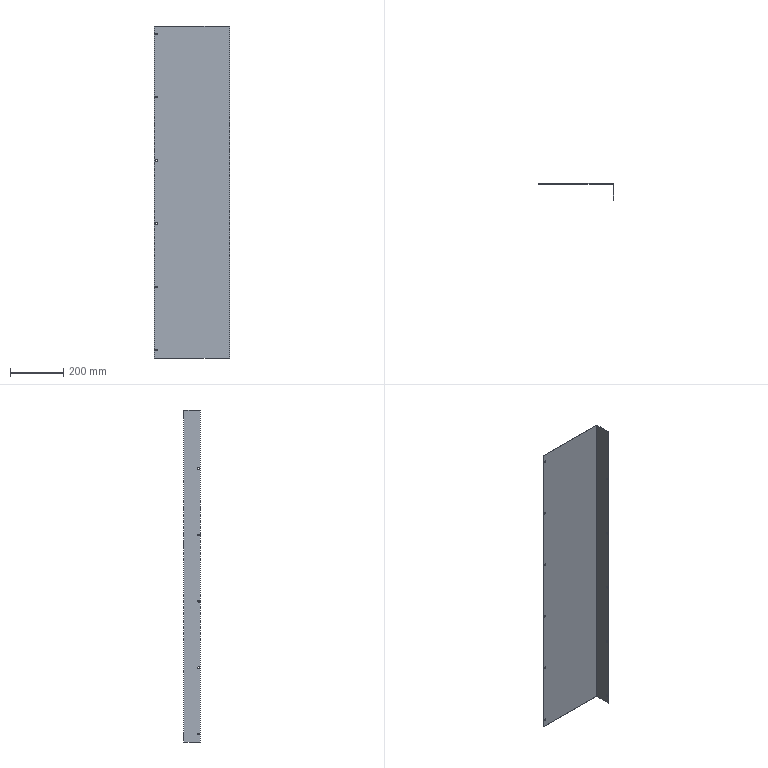Part | SolidWorks | features ICE 2, FlatPattern 1, SMBaseFlange 1, SheetMetal 1 | 1 solid | 69 faces | box 283.5 x 64 x 1250 mm | volume 432234 mm3 | cylinder 35 | plane 34 | commonest cylinder face diameters 6 x33 0.4 x1 2.4 x1